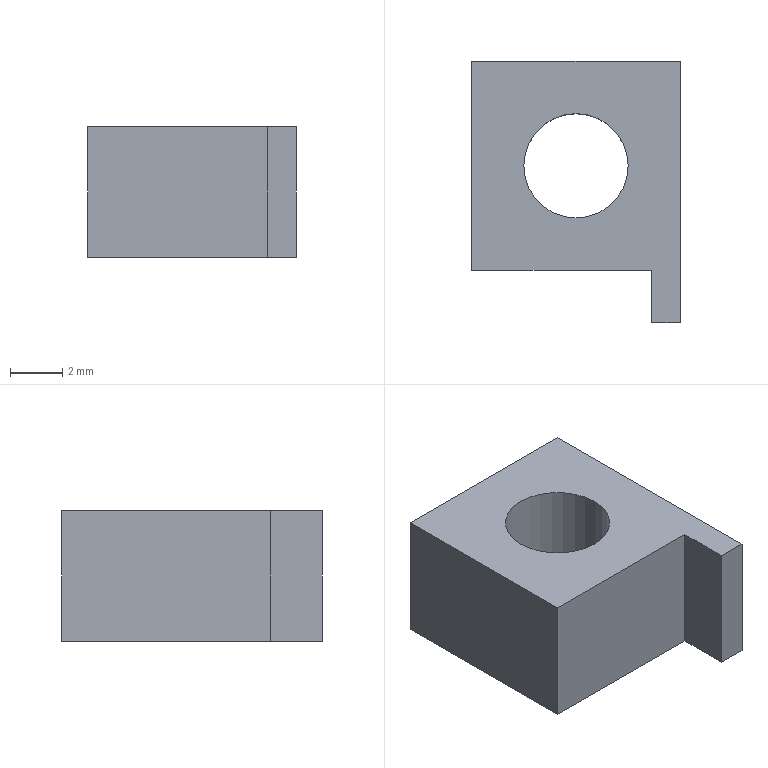Part | NX | 1 solid | 10 faces | box 8 x 10 x 5 mm | volume 268.168 mm3 | plane 8 | cylinder 2 | commonest cylinder face diameters 4 x2
STEP:
#1=CARTESIAN_POINT('',(6.9,0.,0.));
#2=VERTEX_POINT('',#1);
#3=CARTESIAN_POINT('',(6.9,2.,0.));
#4=VERTEX_POINT('',#3);
#5=CARTESIAN_POINT('',(6.9,0.,0.));
#6=DIRECTION('',(0.,1.,0.));
#7=VECTOR('',#6,1000.);
#8=LINE('',#5,#7);
#9=EDGE_CURVE('',#2,#4,#8,.T.);
#10=ORIENTED_EDGE('',*,*,#9,.T.);
#11=CARTESIAN_POINT('',(0.,2.,0.));
#12=VERTEX_POINT('',#11);
#13=CARTESIAN_POINT('',(0.,2.,0.));
#14=DIRECTION('',(1.,0.,0.));
#15=VECTOR('',#14,1000.);
#16=LINE('',#13,#15);
#17=EDGE_CURVE('',#12,#4,#16,.T.);
#18=ORIENTED_EDGE('',*,*,#17,.F.);
#19=CARTESIAN_POINT('',(0.,10.,0.));
#20=VERTEX_POINT('',#19);
#21=CARTESIAN_POINT('',(0.,0.,0.));
#22=DIRECTION('',(0.,1.,0.));
#23=VECTOR('',#22,1000.);
#24=LINE('',#21,#23);
#25=EDGE_CURVE('',#12,#20,#24,.T.);
#26=ORIENTED_EDGE('',*,*,#25,.T.);
#27=CARTESIAN_POINT('',(8.,10.,0.));
#28=VERTEX_POINT('',#27);
#29=CARTESIAN_POINT('',(0.,10.,0.));
#30=DIRECTION('',(1.,0.,0.));
#31=VECTOR('',#30,1000.);
#32=LINE('',#29,#31);
#33=EDGE_CURVE('',#20,#28,#32,.T.);
#34=ORIENTED_EDGE('',*,*,#33,.T.);
#35=CARTESIAN_POINT('',(8.,0.,0.));
#36=VERTEX_POINT('',#35);
#37=CARTESIAN_POINT('',(8.,0.,0.));
#38=DIRECTION('',(0.,-1.,0.));
#39=VECTOR('',#38,1000.);
#40=LINE('',#37,#39);
#41=EDGE_CURVE('',#28,#36,#40,.T.);
#42=ORIENTED_EDGE('',*,*,#41,.T.);
#43=CARTESIAN_POINT('',(0.,0.,0.));
#44=DIRECTION('',(-1.,0.,0.));
#45=VECTOR('',#44,1000.);
#46=LINE('',#43,#45);
#47=EDGE_CURVE('',#36,#2,#46,.T.);
#48=ORIENTED_EDGE('',*,*,#47,.T.);
#49=EDGE_LOOP('',(#10,#18,#26,#34,#42,#48));
#50=FACE_BOUND('',#49,.T.);
#51=CARTESIAN_POINT('',(6.,6.,0.));
#52=VERTEX_POINT('',#51);
#53=CARTESIAN_POINT('',(2.,6.,0.));
#54=VERTEX_POINT('',#53);
#55=CARTESIAN_POINT('',(4.,6.,0.));
#56=DIRECTION('',(0.,0.,-1.));
#57=DIRECTION('',(-1.,0.,0.));
#58=AXIS2_PLACEMENT_3D('',#55,#56,#57);
#59=CIRCLE('',#58,2.);
#60=EDGE_CURVE('',#52,#54,#59,.T.);
#61=ORIENTED_EDGE('',*,*,#60,.F.);
#62=CARTESIAN_POINT('',(4.,6.,0.));
#63=DIRECTION('',(0.,0.,-1.));
#64=DIRECTION('',(-1.,0.,0.));
#65=AXIS2_PLACEMENT_3D('',#62,#63,#64);
#66=CIRCLE('',#65,2.);
#67=EDGE_CURVE('',#54,#52,#66,.T.);
#68=ORIENTED_EDGE('',*,*,#67,.F.);
#69=EDGE_LOOP('',(#61,#68));
#70=FACE_BOUND('',#69,.T.);
#71=CARTESIAN_POINT('',(0.,0.,0.));
#72=DIRECTION('',(0.,0.,1.));
#73=DIRECTION('',(1.,0.,0.));
#74=AXIS2_PLACEMENT_3D('',#71,#72,#73);
#75=PLANE('',#74);
#76=ADVANCED_FACE('',(#50,#70),#75,.F.);
#77=ORIENTED_EDGE('',*,*,#9,.F.);
#78=CARTESIAN_POINT('',(6.9,0.,5.));
#79=VERTEX_POINT('',#78);
#80=CARTESIAN_POINT('',(6.9,0.,0.));
#81=DIRECTION('',(0.,0.,1.));
#82=VECTOR('',#81,1000.);
#83=LINE('',#80,#82);
#84=EDGE_CURVE('',#2,#79,#83,.T.);
#85=ORIENTED_EDGE('',*,*,#84,.T.);
#86=CARTESIAN_POINT('',(6.9,2.,5.));
#87=VERTEX_POINT('',#86);
#88=CARTESIAN_POINT('',(6.9,0.,5.));
#89=DIRECTION('',(0.,1.,0.));
#90=VECTOR('',#89,1000.);
#91=LINE('',#88,#90);
#92=EDGE_CURVE('',#79,#87,#91,.T.);
#93=ORIENTED_EDGE('',*,*,#92,.T.);
#94=CARTESIAN_POINT('',(6.9,2.,0.));
#95=DIRECTION('',(0.,0.,-1.));
#96=VECTOR('',#95,1000.);
#97=LINE('',#94,#96);
#98=EDGE_CURVE('',#87,#4,#97,.T.);
#99=ORIENTED_EDGE('',*,*,#98,.T.);
#100=EDGE_LOOP('',(#77,#85,#93,#99));
#101=FACE_BOUND('',#100,.T.);
#102=CARTESIAN_POINT('',(6.9,0.,5.));
#103=DIRECTION('',(1.,0.,0.));
#104=DIRECTION('',(0.,1.,0.));
#105=AXIS2_PLACEMENT_3D('',#102,#103,#104);
#106=PLANE('',#105);
#107=ADVANCED_FACE('',(#101),#106,.F.);
#108=ORIENTED_EDGE('',*,*,#17,.T.);
#109=ORIENTED_EDGE('',*,*,#98,.F.);
#110=CARTESIAN_POINT('',(0.,2.,5.));
#111=VERTEX_POINT('',#110);
#112=CARTESIAN_POINT('',(0.,2.,5.));
#113=DIRECTION('',(1.,0.,0.));
#114=VECTOR('',#113,1000.);
#115=LINE('',#112,#114);
#116=EDGE_CURVE('',#111,#87,#115,.T.);
#117=ORIENTED_EDGE('',*,*,#116,.F.);
#118=CARTESIAN_POINT('',(0.,2.,0.));
#119=DIRECTION('',(0.,0.,-1.));
#120=VECTOR('',#119,1000.);
#121=LINE('',#118,#120);
#122=EDGE_CURVE('',#111,#12,#121,.T.);
#123=ORIENTED_EDGE('',*,*,#122,.T.);
#124=EDGE_LOOP('',(#108,#109,#117,#123));
#125=FACE_BOUND('',#124,.T.);
#126=CARTESIAN_POINT('',(7.,2.,5.));
#127=DIRECTION('',(0.,1.,0.));
#128=DIRECTION('',(1.,0.,0.));
#129=AXIS2_PLACEMENT_3D('',#126,#127,#128);
#130=PLANE('',#129);
#131=ADVANCED_FACE('',(#125),#130,.F.);
#132=ORIENTED_EDGE('',*,*,#122,.F.);
#133=CARTESIAN_POINT('',(0.,10.,5.));
#134=VERTEX_POINT('',#133);
#135=CARTESIAN_POINT('',(0.,0.,5.));
#136=DIRECTION('',(0.,1.,0.));
#137=VECTOR('',#136,1000.);
#138=LINE('',#135,#137);
#139=EDGE_CURVE('',#111,#134,#138,.T.);
#140=ORIENTED_EDGE('',*,*,#139,.T.);
#141=CARTESIAN_POINT('',(0.,10.,5.));
#142=DIRECTION('',(0.,0.,-1.));
#143=VECTOR('',#142,1000.);
#144=LINE('',#141,#143);
#145=EDGE_CURVE('',#134,#20,#144,.T.);
#146=ORIENTED_EDGE('',*,*,#145,.T.);
#147=ORIENTED_EDGE('',*,*,#25,.F.);
#148=EDGE_LOOP('',(#132,#140,#146,#147));
#149=FACE_BOUND('',#148,.T.);
#150=CARTESIAN_POINT('',(0.,10.,0.));
#151=DIRECTION('',(-1.,0.,0.));
#152=DIRECTION('',(0.,0.,1.));
#153=AXIS2_PLACEMENT_3D('',#150,#151,#152);
#154=PLANE('',#153);
#155=ADVANCED_FACE('',(#149),#154,.T.);
#156=ORIENTED_EDGE('',*,*,#33,.F.);
#157=ORIENTED_EDGE('',*,*,#145,.F.);
#158=CARTESIAN_POINT('',(8.,10.,5.));
#159=VERTEX_POINT('',#158);
#160=CARTESIAN_POINT('',(0.,10.,5.));
#161=DIRECTION('',(1.,0.,0.));
#162=VECTOR('',#161,1000.);
#163=LINE('',#160,#162);
#164=EDGE_CURVE('',#134,#159,#163,.T.);
#165=ORIENTED_EDGE('',*,*,#164,.T.);
#166=CARTESIAN_POINT('',(8.,10.,5.));
#167=DIRECTION('',(0.,0.,-1.));
#168=VECTOR('',#167,1000.);
#169=LINE('',#166,#168);
#170=EDGE_CURVE('',#159,#28,#169,.T.);
#171=ORIENTED_EDGE('',*,*,#170,.T.);
#172=EDGE_LOOP('',(#156,#157,#165,#171));
#173=FACE_BOUND('',#172,.T.);
#174=CARTESIAN_POINT('',(8.,10.,0.));
#175=DIRECTION('',(0.,1.,0.));
#176=DIRECTION('',(1.,0.,0.));
#177=AXIS2_PLACEMENT_3D('',#174,#175,#176);
#178=PLANE('',#177);
#179=ADVANCED_FACE('',(#173),#178,.T.);
#180=ORIENTED_EDGE('',*,*,#41,.F.);
#181=ORIENTED_EDGE('',*,*,#170,.F.);
#182=CARTESIAN_POINT('',(8.,0.,5.));
#183=VERTEX_POINT('',#182);
#184=CARTESIAN_POINT('',(8.,0.,5.));
#185=DIRECTION('',(0.,-1.,0.));
#186=VECTOR('',#185,1000.);
#187=LINE('',#184,#186);
#188=EDGE_CURVE('',#159,#183,#187,.T.);
#189=ORIENTED_EDGE('',*,*,#188,.T.);
#190=CARTESIAN_POINT('',(8.,0.,0.));
#191=DIRECTION('',(0.,0.,-1.));
#192=VECTOR('',#191,1000.);
#193=LINE('',#190,#192);
#194=EDGE_CURVE('',#183,#36,#193,.T.);
#195=ORIENTED_EDGE('',*,*,#194,.T.);
#196=EDGE_LOOP('',(#180,#181,#189,#195));
#197=FACE_BOUND('',#196,.T.);
#198=CARTESIAN_POINT('',(8.,0.,0.));
#199=DIRECTION('',(1.,0.,0.));
#200=DIRECTION('',(0.,1.,0.));
#201=AXIS2_PLACEMENT_3D('',#198,#199,#200);
#202=PLANE('',#201);
#203=ADVANCED_FACE('',(#197),#202,.T.);
#204=ORIENTED_EDGE('',*,*,#84,.F.);
#205=ORIENTED_EDGE('',*,*,#47,.F.);
#206=ORIENTED_EDGE('',*,*,#194,.F.);
#207=CARTESIAN_POINT('',(0.,0.,5.));
#208=DIRECTION('',(-1.,0.,0.));
#209=VECTOR('',#208,1000.);
#210=LINE('',#207,#209);
#211=EDGE_CURVE('',#183,#79,#210,.T.);
#212=ORIENTED_EDGE('',*,*,#211,.T.);
#213=EDGE_LOOP('',(#204,#205,#206,#212));
#214=FACE_BOUND('',#213,.T.);
#215=CARTESIAN_POINT('',(0.,0.,0.));
#216=DIRECTION('',(0.,-1.,0.));
#217=DIRECTION('',(0.,0.,-1.));
#218=AXIS2_PLACEMENT_3D('',#215,#216,#217);
#219=PLANE('',#218);
#220=ADVANCED_FACE('',(#214),#219,.T.);
#221=ORIENTED_EDGE('',*,*,#92,.F.);
#222=ORIENTED_EDGE('',*,*,#211,.F.);
#223=ORIENTED_EDGE('',*,*,#188,.F.);
#224=ORIENTED_EDGE('',*,*,#164,.F.);
#225=ORIENTED_EDGE('',*,*,#139,.F.);
#226=ORIENTED_EDGE('',*,*,#116,.T.);
#227=EDGE_LOOP('',(#221,#222,#223,#224,#225,#226));
#228=FACE_BOUND('',#227,.T.);
#229=CARTESIAN_POINT('',(6.,6.,5.));
#230=VERTEX_POINT('',#229);
#231=CARTESIAN_POINT('',(2.,6.,5.));
#232=VERTEX_POINT('',#231);
#233=CARTESIAN_POINT('',(4.,6.,5.));
#234=DIRECTION('',(0.,0.,-1.));
#235=DIRECTION('',(-1.,0.,0.));
#236=AXIS2_PLACEMENT_3D('',#233,#234,#235);
#237=CIRCLE('',#236,2.);
#238=EDGE_CURVE('',#230,#232,#237,.T.);
#239=ORIENTED_EDGE('',*,*,#238,.T.);
#240=CARTESIAN_POINT('',(4.,6.,5.));
#241=DIRECTION('',(0.,0.,-1.));
#242=DIRECTION('',(-1.,0.,0.));
#243=AXIS2_PLACEMENT_3D('',#240,#241,#242);
#244=CIRCLE('',#243,2.);
#245=EDGE_CURVE('',#232,#230,#244,.T.);
#246=ORIENTED_EDGE('',*,*,#245,.T.);
#247=EDGE_LOOP('',(#239,#246));
#248=FACE_BOUND('',#247,.T.);
#249=CARTESIAN_POINT('',(0.,0.,5.));
#250=DIRECTION('',(0.,0.,1.));
#251=DIRECTION('',(1.,0.,0.));
#252=AXIS2_PLACEMENT_3D('',#249,#250,#251);
#253=PLANE('',#252);
#254=ADVANCED_FACE('',(#228,#248),#253,.T.);
#255=ORIENTED_EDGE('',*,*,#238,.F.);
#256=CARTESIAN_POINT('',(6.,6.,5.));
#257=DIRECTION('',(0.,0.,-1.));
#258=VECTOR('',#257,1000.);
#259=LINE('',#256,#258);
#260=EDGE_CURVE('',#52,#230,#259,.F.);
#261=ORIENTED_EDGE('',*,*,#260,.F.);
#262=ORIENTED_EDGE('',*,*,#60,.T.);
#263=CARTESIAN_POINT('',(2.,6.,5.));
#264=DIRECTION('',(0.,0.,-1.));
#265=VECTOR('',#264,1000.);
#266=LINE('',#263,#265);
#267=EDGE_CURVE('',#54,#232,#266,.F.);
#268=ORIENTED_EDGE('',*,*,#267,.T.);
#269=EDGE_LOOP('',(#255,#261,#262,#268));
#270=FACE_BOUND('',#269,.T.);
#271=CARTESIAN_POINT('',(4.,6.,5.));
#272=DIRECTION('',(0.,0.,-1.));
#273=DIRECTION('',(-1.,0.,0.));
#274=AXIS2_PLACEMENT_3D('',#271,#272,#273);
#275=CYLINDRICAL_SURFACE('',#274,2.);
#276=ADVANCED_FACE('',(#270),#275,.F.);
#277=ORIENTED_EDGE('',*,*,#267,.F.);
#278=ORIENTED_EDGE('',*,*,#67,.T.);
#279=ORIENTED_EDGE('',*,*,#260,.T.);
#280=ORIENTED_EDGE('',*,*,#245,.F.);
#281=EDGE_LOOP('',(#277,#278,#279,#280));
#282=FACE_BOUND('',#281,.T.);
#283=CARTESIAN_POINT('',(4.,6.,5.));
#284=DIRECTION('',(0.,0.,-1.));
#285=DIRECTION('',(-1.,0.,0.));
#286=AXIS2_PLACEMENT_3D('',#283,#284,#285);
#287=CYLINDRICAL_SURFACE('',#286,2.);
#288=ADVANCED_FACE('',(#282),#287,.F.);
#289=CLOSED_SHELL('',(#76,#107,#131,#155,#179,#203,#220,#254,#276,#288));
#290=MANIFOLD_SOLID_BREP('',#289);
#291=(LENGTH_UNIT()NAMED_UNIT(*)SI_UNIT(.MILLI.,.METRE.));
#292=UNCERTAINTY_MEASURE_WITH_UNIT(LENGTH_MEASURE(0.00001),#291,'','');
#293=(NAMED_UNIT(*)PLANE_ANGLE_UNIT()SI_UNIT($,.RADIAN.));
#294=(NAMED_UNIT(*)SI_UNIT($,.STERADIAN.)SOLID_ANGLE_UNIT());
#295=(GEOMETRIC_REPRESENTATION_CONTEXT(3)GLOBAL_UNCERTAINTY_ASSIGNED_CONTEXT((#292))GLOBAL_UNIT_ASSIGNED_CONTEXT((#291,#293,#294))REPRESENTATION_CONTEXT('',''));
#296=ADVANCED_BREP_SHAPE_REPRESENTATION('',(#290),#295);